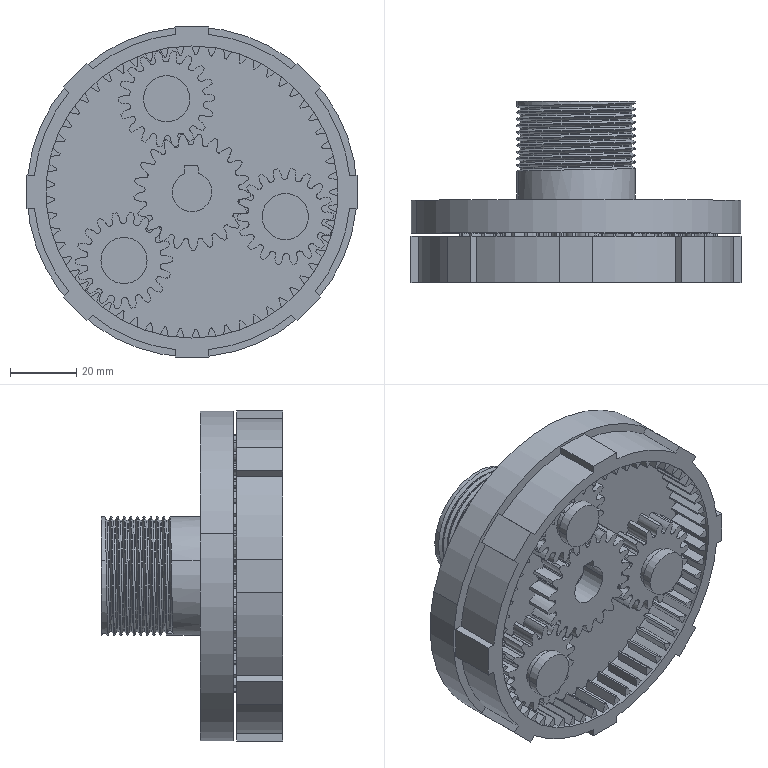Part | SolidWorks | features CompositeCurve 16 | 9 solids | 723 faces | box 100 x 55 x 100 mm | volume 136312 mm3 | cylinder 280 | spline 267 | plane 176 | commonest cylinder face diameters 29.25 x57 83.25 x57 22.5 x54 12 x26 36 x22 28.5 x21